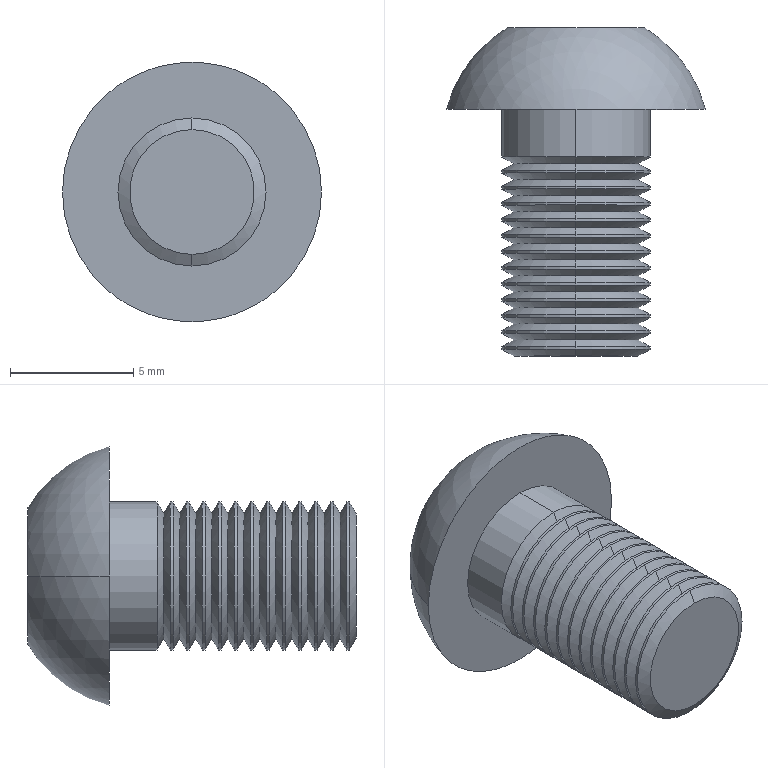Part | SolidWorks | features BaseBody 1 | 1 solid | 93 faces | box 10.5 x 13.3 x 10.5 mm | volume 422.27 mm3 | cone 50 | cylinder 26 | plane 15 | sphere 2 | commonest cylinder face diameters 6 x26